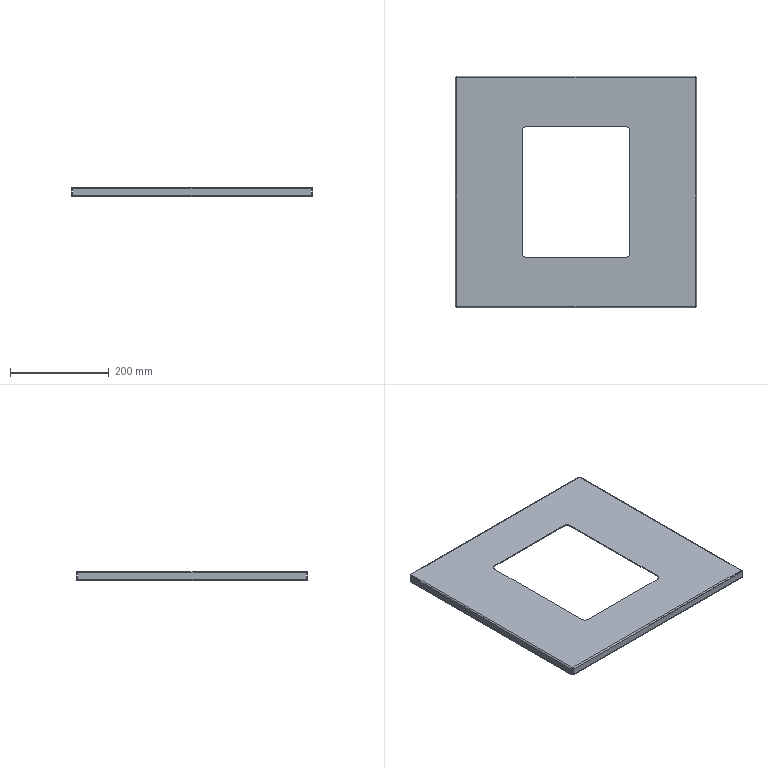Part | STEP file | MYT-A01-P23 | 1 solid | 78 faces | box 489 x 469 x 18 mm | volume 480238 mm3 | plane 42 | cylinder 20 | spline 16 | commonest cylinder face diameters 1.473 x8 5.473 x8 20 x4